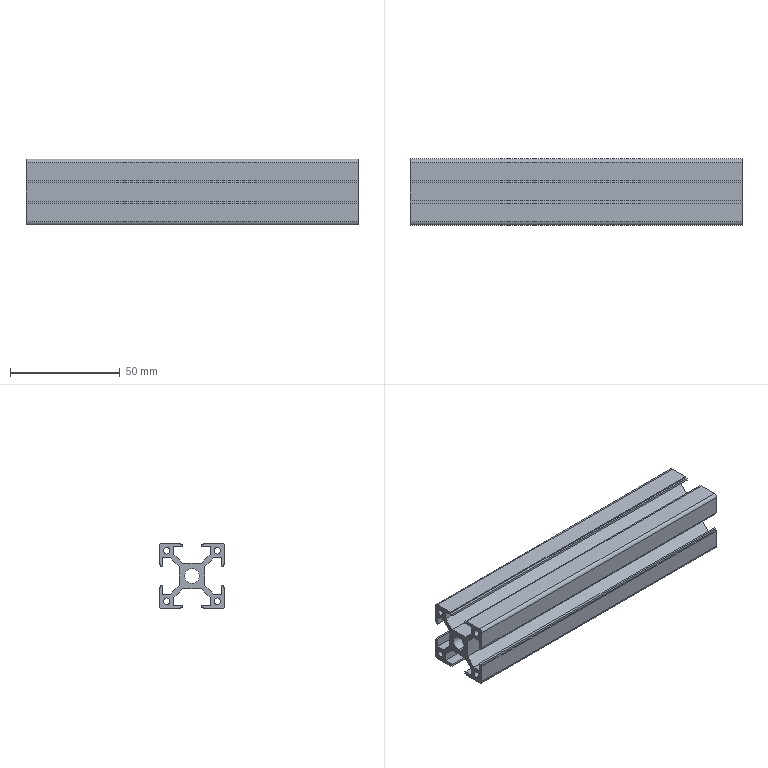Part | STEP file | 001-004-Feeding mechanism support profile_default<machined> | 1 solid | 76 faces | box 151 x 30 x 30 mm | volume 50748 mm3 | plane 62 | cylinder 14 | commonest cylinder face diameters 3 x12 6.8 x2